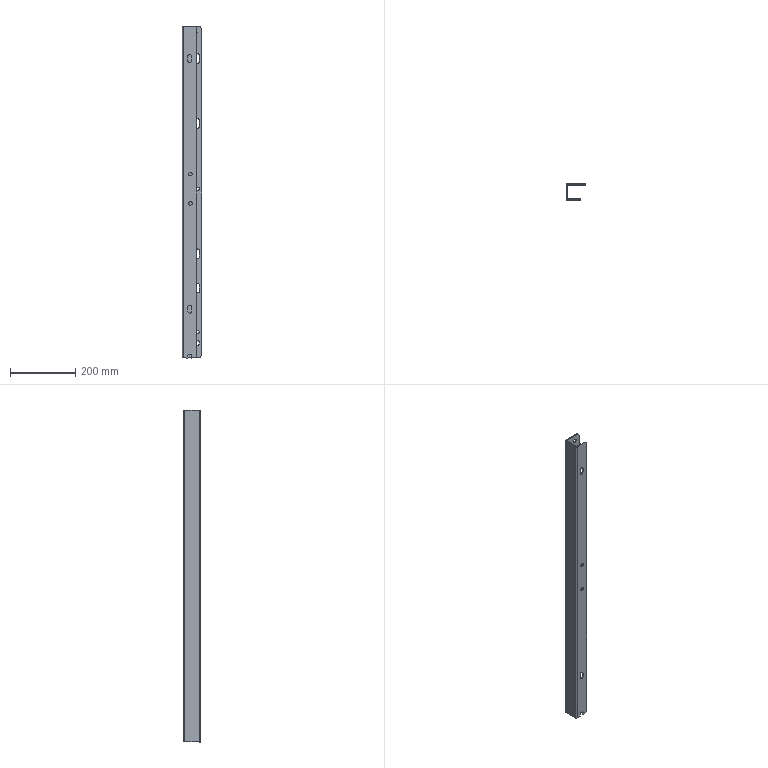Part | 1 solid | 70 faces | box 60 x 50 x 1020 mm | volume 444037 mm3 | cylinder 35 | plane 35 | commonest cylinder face diameters 10 x14 12 x9 11 x4 24 x4 0.4 x2 6.4 x2